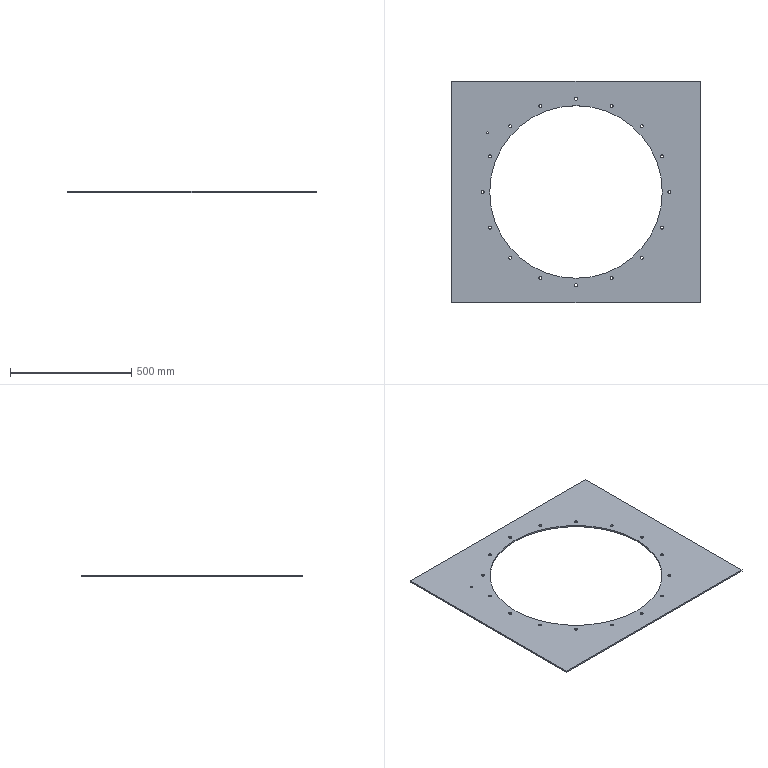Part | STEP file | 750078200 | 1 solid | 42 faces | box 1025 x 915 x 6 mm | volume 3220443 mm3 | cylinder 36 | plane 6 | commonest cylinder face diameters 12 x32 8.2 x2 713 x2
STEP:
#1=CARTESIAN_POINT('',(-356.5,0.,0.));
#2=VERTEX_POINT('',#1);
#3=CARTESIAN_POINT('',(356.5,0.,0.));
#4=VERTEX_POINT('',#3);
#5=CARTESIAN_POINT('',(0.,0.,0.));
#6=DIRECTION('',(0.,0.,1.));
#7=DIRECTION('',(1.,0.,0.));
#8=AXIS2_PLACEMENT_3D('',#5,#6,#7);
#9=CIRCLE('',#8,356.5);
#10=EDGE_CURVE('',#2,#4,#9,.T.);
#11=ORIENTED_EDGE('',*,*,#10,.F.);
#12=CARTESIAN_POINT('',(-356.5,0.,6.));
#13=VERTEX_POINT('',#12);
#14=CARTESIAN_POINT('',(-356.5,0.,-1368.004));
#15=DIRECTION('',(0.,0.,1.));
#16=VECTOR('',#15,1000.);
#17=LINE('',#14,#16);
#18=EDGE_CURVE('',#2,#13,#17,.T.);
#19=ORIENTED_EDGE('',*,*,#18,.T.);
#20=CARTESIAN_POINT('',(356.5,0.,6.));
#21=VERTEX_POINT('',#20);
#22=CARTESIAN_POINT('',(0.,0.,6.));
#23=DIRECTION('',(0.,0.,-1.));
#24=DIRECTION('',(1.,0.,0.));
#25=AXIS2_PLACEMENT_3D('',#22,#23,#24);
#26=CIRCLE('',#25,356.5);
#27=EDGE_CURVE('',#21,#13,#26,.T.);
#28=ORIENTED_EDGE('',*,*,#27,.F.);
#29=CARTESIAN_POINT('',(356.5,0.,-1368.004));
#30=DIRECTION('',(0.,0.,1.));
#31=VECTOR('',#30,1000.);
#32=LINE('',#29,#31);
#33=EDGE_CURVE('',#4,#21,#32,.T.);
#34=ORIENTED_EDGE('',*,*,#33,.F.);
#35=EDGE_LOOP('',(#11,#19,#28,#34));
#36=FACE_OUTER_BOUND('',#35,.T.);
#37=CARTESIAN_POINT('',(0.,0.,-1368.004));
#38=DIRECTION('',(0.,0.,1.));
#39=DIRECTION('',(1.,0.,0.));
#40=AXIS2_PLACEMENT_3D('',#37,#38,#39);
#41=CYLINDRICAL_SURFACE('',#40,356.5);
#42=ADVANCED_FACE('',(#36),#41,.F.);
#43=CARTESIAN_POINT('',(379.,0.,0.));
#44=VERTEX_POINT('',#43);
#45=CARTESIAN_POINT('',(391.,0.,0.));
#46=VERTEX_POINT('',#45);
#47=CARTESIAN_POINT('',(385.,0.,0.));
#48=DIRECTION('',(0.,0.,1.));
#49=DIRECTION('',(1.,0.,0.));
#50=AXIS2_PLACEMENT_3D('',#47,#48,#49);
#51=CIRCLE('',#50,6.);
#52=EDGE_CURVE('',#44,#46,#51,.T.);
#53=ORIENTED_EDGE('',*,*,#52,.F.);
#54=CARTESIAN_POINT('',(379.,0.,6.));
#55=VERTEX_POINT('',#54);
#56=CARTESIAN_POINT('',(379.,0.,-1368.004));
#57=DIRECTION('',(0.,0.,1.));
#58=VECTOR('',#57,1000.);
#59=LINE('',#56,#58);
#60=EDGE_CURVE('',#44,#55,#59,.T.);
#61=ORIENTED_EDGE('',*,*,#60,.T.);
#62=CARTESIAN_POINT('',(391.,0.,6.));
#63=VERTEX_POINT('',#62);
#64=CARTESIAN_POINT('',(385.,0.,6.));
#65=DIRECTION('',(0.,0.,-1.));
#66=DIRECTION('',(1.,0.,0.));
#67=AXIS2_PLACEMENT_3D('',#64,#65,#66);
#68=CIRCLE('',#67,6.);
#69=EDGE_CURVE('',#63,#55,#68,.T.);
#70=ORIENTED_EDGE('',*,*,#69,.F.);
#71=CARTESIAN_POINT('',(391.,0.,-1368.004));
#72=DIRECTION('',(0.,0.,1.));
#73=VECTOR('',#72,1000.);
#74=LINE('',#71,#73);
#75=EDGE_CURVE('',#46,#63,#74,.T.);
#76=ORIENTED_EDGE('',*,*,#75,.F.);
#77=EDGE_LOOP('',(#53,#61,#70,#76));
#78=FACE_OUTER_BOUND('',#77,.T.);
#79=CARTESIAN_POINT('',(385.,0.,-1368.004));
#80=DIRECTION('',(0.,0.,1.));
#81=DIRECTION('',(1.,0.,0.));
#82=AXIS2_PLACEMENT_3D('',#79,#80,#81);
#83=CYLINDRICAL_SURFACE('',#82,6.);
#84=ADVANCED_FACE('',(#78),#83,.F.);
#85=CARTESIAN_POINT('',(349.694,-147.333,0.));
#86=VERTEX_POINT('',#85);
#87=CARTESIAN_POINT('',(361.694,-147.333,0.));
#88=VERTEX_POINT('',#87);
#89=CARTESIAN_POINT('',(355.694,-147.333,0.));
#90=DIRECTION('',(0.,0.,1.));
#91=DIRECTION('',(1.,0.,0.));
#92=AXIS2_PLACEMENT_3D('',#89,#90,#91);
#93=CIRCLE('',#92,6.);
#94=EDGE_CURVE('',#86,#88,#93,.T.);
#95=ORIENTED_EDGE('',*,*,#94,.F.);
#96=CARTESIAN_POINT('',(349.694,-147.333,6.));
#97=VERTEX_POINT('',#96);
#98=CARTESIAN_POINT('',(349.694,-147.333,-1368.004));
#99=DIRECTION('',(0.,0.,1.));
#100=VECTOR('',#99,1000.);
#101=LINE('',#98,#100);
#102=EDGE_CURVE('',#86,#97,#101,.T.);
#103=ORIENTED_EDGE('',*,*,#102,.T.);
#104=CARTESIAN_POINT('',(361.694,-147.333,6.));
#105=VERTEX_POINT('',#104);
#106=CARTESIAN_POINT('',(355.694,-147.333,6.));
#107=DIRECTION('',(0.,0.,-1.));
#108=DIRECTION('',(1.,0.,0.));
#109=AXIS2_PLACEMENT_3D('',#106,#107,#108);
#110=CIRCLE('',#109,6.);
#111=EDGE_CURVE('',#105,#97,#110,.T.);
#112=ORIENTED_EDGE('',*,*,#111,.F.);
#113=CARTESIAN_POINT('',(361.694,-147.333,-1368.004));
#114=DIRECTION('',(0.,0.,1.));
#115=VECTOR('',#114,1000.);
#116=LINE('',#113,#115);
#117=EDGE_CURVE('',#88,#105,#116,.T.);
#118=ORIENTED_EDGE('',*,*,#117,.F.);
#119=EDGE_LOOP('',(#95,#103,#112,#118));
#120=FACE_OUTER_BOUND('',#119,.T.);
#121=CARTESIAN_POINT('',(355.694,-147.333,-1368.004));
#122=DIRECTION('',(0.,0.,1.));
#123=DIRECTION('',(1.,0.,0.));
#124=AXIS2_PLACEMENT_3D('',#121,#122,#123);
#125=CYLINDRICAL_SURFACE('',#124,6.);
#126=ADVANCED_FACE('',(#120),#125,.F.);
#127=CARTESIAN_POINT('',(349.694,147.333,0.));
#128=VERTEX_POINT('',#127);
#129=CARTESIAN_POINT('',(361.694,147.333,0.));
#130=VERTEX_POINT('',#129);
#131=CARTESIAN_POINT('',(355.694,147.333,0.));
#132=DIRECTION('',(0.,0.,1.));
#133=DIRECTION('',(1.,0.,0.));
#134=AXIS2_PLACEMENT_3D('',#131,#132,#133);
#135=CIRCLE('',#134,6.);
#136=EDGE_CURVE('',#128,#130,#135,.T.);
#137=ORIENTED_EDGE('',*,*,#136,.F.);
#138=CARTESIAN_POINT('',(349.694,147.333,6.));
#139=VERTEX_POINT('',#138);
#140=CARTESIAN_POINT('',(349.694,147.333,-1368.004));
#141=DIRECTION('',(0.,0.,1.));
#142=VECTOR('',#141,1000.);
#143=LINE('',#140,#142);
#144=EDGE_CURVE('',#128,#139,#143,.T.);
#145=ORIENTED_EDGE('',*,*,#144,.T.);
#146=CARTESIAN_POINT('',(361.694,147.333,6.));
#147=VERTEX_POINT('',#146);
#148=CARTESIAN_POINT('',(355.694,147.333,6.));
#149=DIRECTION('',(0.,0.,-1.));
#150=DIRECTION('',(1.,0.,0.));
#151=AXIS2_PLACEMENT_3D('',#148,#149,#150);
#152=CIRCLE('',#151,6.);
#153=EDGE_CURVE('',#147,#139,#152,.T.);
#154=ORIENTED_EDGE('',*,*,#153,.F.);
#155=CARTESIAN_POINT('',(361.694,147.333,-1368.004));
#156=DIRECTION('',(0.,0.,1.));
#157=VECTOR('',#156,1000.);
#158=LINE('',#155,#157);
#159=EDGE_CURVE('',#130,#147,#158,.T.);
#160=ORIENTED_EDGE('',*,*,#159,.F.);
#161=EDGE_LOOP('',(#137,#145,#154,#160));
#162=FACE_OUTER_BOUND('',#161,.T.);
#163=CARTESIAN_POINT('',(355.694,147.333,-1368.004));
#164=DIRECTION('',(0.,0.,1.));
#165=DIRECTION('',(1.,0.,0.));
#166=AXIS2_PLACEMENT_3D('',#163,#164,#165);
#167=CYLINDRICAL_SURFACE('',#166,6.);
#168=ADVANCED_FACE('',(#162),#167,.F.);
#169=CARTESIAN_POINT('',(266.236,272.236,0.));
#170=VERTEX_POINT('',#169);
#171=CARTESIAN_POINT('',(278.236,272.236,0.));
#172=VERTEX_POINT('',#171);
#173=CARTESIAN_POINT('',(272.236,272.236,0.));
#174=DIRECTION('',(0.,0.,1.));
#175=DIRECTION('',(1.,0.,0.));
#176=AXIS2_PLACEMENT_3D('',#173,#174,#175);
#177=CIRCLE('',#176,6.);
#178=EDGE_CURVE('',#170,#172,#177,.T.);
#179=ORIENTED_EDGE('',*,*,#178,.F.);
#180=CARTESIAN_POINT('',(266.236,272.236,6.));
#181=VERTEX_POINT('',#180);
#182=CARTESIAN_POINT('',(266.236,272.236,-1368.004));
#183=DIRECTION('',(0.,0.,1.));
#184=VECTOR('',#183,1000.);
#185=LINE('',#182,#184);
#186=EDGE_CURVE('',#170,#181,#185,.T.);
#187=ORIENTED_EDGE('',*,*,#186,.T.);
#188=CARTESIAN_POINT('',(278.236,272.236,6.));
#189=VERTEX_POINT('',#188);
#190=CARTESIAN_POINT('',(272.236,272.236,6.));
#191=DIRECTION('',(0.,0.,-1.));
#192=DIRECTION('',(1.,0.,0.));
#193=AXIS2_PLACEMENT_3D('',#190,#191,#192);
#194=CIRCLE('',#193,6.);
#195=EDGE_CURVE('',#189,#181,#194,.T.);
#196=ORIENTED_EDGE('',*,*,#195,.F.);
#197=CARTESIAN_POINT('',(278.236,272.236,-1368.004));
#198=DIRECTION('',(0.,0.,1.));
#199=VECTOR('',#198,1000.);
#200=LINE('',#197,#199);
#201=EDGE_CURVE('',#172,#189,#200,.T.);
#202=ORIENTED_EDGE('',*,*,#201,.F.);
#203=EDGE_LOOP('',(#179,#187,#196,#202));
#204=FACE_OUTER_BOUND('',#203,.T.);
#205=CARTESIAN_POINT('',(272.236,272.236,-1368.004));
#206=DIRECTION('',(0.,0.,1.));
#207=DIRECTION('',(1.,0.,0.));
#208=AXIS2_PLACEMENT_3D('',#205,#206,#207);
#209=CYLINDRICAL_SURFACE('',#208,6.);
#210=ADVANCED_FACE('',(#204),#209,.F.);
#211=CARTESIAN_POINT('',(266.236,-272.236,0.));
#212=VERTEX_POINT('',#211);
#213=CARTESIAN_POINT('',(278.236,-272.236,0.));
#214=VERTEX_POINT('',#213);
#215=CARTESIAN_POINT('',(272.236,-272.236,0.));
#216=DIRECTION('',(0.,0.,1.));
#217=DIRECTION('',(1.,0.,0.));
#218=AXIS2_PLACEMENT_3D('',#215,#216,#217);
#219=CIRCLE('',#218,6.);
#220=EDGE_CURVE('',#212,#214,#219,.T.);
#221=ORIENTED_EDGE('',*,*,#220,.F.);
#222=CARTESIAN_POINT('',(266.236,-272.236,6.));
#223=VERTEX_POINT('',#222);
#224=CARTESIAN_POINT('',(266.236,-272.236,-1368.004));
#225=DIRECTION('',(0.,0.,1.));
#226=VECTOR('',#225,1000.);
#227=LINE('',#224,#226);
#228=EDGE_CURVE('',#212,#223,#227,.T.);
#229=ORIENTED_EDGE('',*,*,#228,.T.);
#230=CARTESIAN_POINT('',(278.236,-272.236,6.));
#231=VERTEX_POINT('',#230);
#232=CARTESIAN_POINT('',(272.236,-272.236,6.));
#233=DIRECTION('',(0.,0.,-1.));
#234=DIRECTION('',(1.,0.,0.));
#235=AXIS2_PLACEMENT_3D('',#232,#233,#234);
#236=CIRCLE('',#235,6.);
#237=EDGE_CURVE('',#231,#223,#236,.T.);
#238=ORIENTED_EDGE('',*,*,#237,.F.);
#239=CARTESIAN_POINT('',(278.236,-272.236,-1368.004));
#240=DIRECTION('',(0.,0.,1.));
#241=VECTOR('',#240,1000.);
#242=LINE('',#239,#241);
#243=EDGE_CURVE('',#214,#231,#242,.T.);
#244=ORIENTED_EDGE('',*,*,#243,.F.);
#245=EDGE_LOOP('',(#221,#229,#238,#244));
#246=FACE_OUTER_BOUND('',#245,.T.);
#247=CARTESIAN_POINT('',(272.236,-272.236,-1368.004));
#248=DIRECTION('',(0.,0.,1.));
#249=DIRECTION('',(1.,0.,0.));
#250=AXIS2_PLACEMENT_3D('',#247,#248,#249);
#251=CYLINDRICAL_SURFACE('',#250,6.);
#252=ADVANCED_FACE('',(#246),#251,.F.);
#253=CARTESIAN_POINT('',(141.333,355.694,0.));
#254=VERTEX_POINT('',#253);
#255=CARTESIAN_POINT('',(153.333,355.694,0.));
#256=VERTEX_POINT('',#255);
#257=CARTESIAN_POINT('',(147.333,355.694,0.));
#258=DIRECTION('',(0.,0.,1.));
#259=DIRECTION('',(1.,0.,0.));
#260=AXIS2_PLACEMENT_3D('',#257,#258,#259);
#261=CIRCLE('',#260,6.);
#262=EDGE_CURVE('',#254,#256,#261,.T.);
#263=ORIENTED_EDGE('',*,*,#262,.F.);
#264=CARTESIAN_POINT('',(141.333,355.694,6.));
#265=VERTEX_POINT('',#264);
#266=CARTESIAN_POINT('',(141.333,355.694,-1368.004));
#267=DIRECTION('',(0.,0.,1.));
#268=VECTOR('',#267,1000.);
#269=LINE('',#266,#268);
#270=EDGE_CURVE('',#254,#265,#269,.T.);
#271=ORIENTED_EDGE('',*,*,#270,.T.);
#272=CARTESIAN_POINT('',(153.333,355.694,6.));
#273=VERTEX_POINT('',#272);
#274=CARTESIAN_POINT('',(147.333,355.694,6.));
#275=DIRECTION('',(0.,0.,-1.));
#276=DIRECTION('',(1.,0.,0.));
#277=AXIS2_PLACEMENT_3D('',#274,#275,#276);
#278=CIRCLE('',#277,6.);
#279=EDGE_CURVE('',#273,#265,#278,.T.);
#280=ORIENTED_EDGE('',*,*,#279,.F.);
#281=CARTESIAN_POINT('',(153.333,355.694,-1368.004));
#282=DIRECTION('',(0.,0.,1.));
#283=VECTOR('',#282,1000.);
#284=LINE('',#281,#283);
#285=EDGE_CURVE('',#256,#273,#284,.T.);
#286=ORIENTED_EDGE('',*,*,#285,.F.);
#287=EDGE_LOOP('',(#263,#271,#280,#286));
#288=FACE_OUTER_BOUND('',#287,.T.);
#289=CARTESIAN_POINT('',(147.333,355.694,-1368.004));
#290=DIRECTION('',(0.,0.,1.));
#291=DIRECTION('',(1.,0.,0.));
#292=AXIS2_PLACEMENT_3D('',#289,#290,#291);
#293=CYLINDRICAL_SURFACE('',#292,6.);
#294=ADVANCED_FACE('',(#288),#293,.F.);
#295=CARTESIAN_POINT('',(141.333,-355.694,0.));
#296=VERTEX_POINT('',#295);
#297=CARTESIAN_POINT('',(153.333,-355.694,0.));
#298=VERTEX_POINT('',#297);
#299=CARTESIAN_POINT('',(147.333,-355.694,0.));
#300=DIRECTION('',(0.,0.,1.));
#301=DIRECTION('',(1.,0.,0.));
#302=AXIS2_PLACEMENT_3D('',#299,#300,#301);
#303=CIRCLE('',#302,6.);
#304=EDGE_CURVE('',#296,#298,#303,.T.);
#305=ORIENTED_EDGE('',*,*,#304,.F.);
#306=CARTESIAN_POINT('',(141.333,-355.694,6.));
#307=VERTEX_POINT('',#306);
#308=CARTESIAN_POINT('',(141.333,-355.694,-1368.004));
#309=DIRECTION('',(0.,0.,1.));
#310=VECTOR('',#309,1000.);
#311=LINE('',#308,#310);
#312=EDGE_CURVE('',#296,#307,#311,.T.);
#313=ORIENTED_EDGE('',*,*,#312,.T.);
#314=CARTESIAN_POINT('',(153.333,-355.694,6.));
#315=VERTEX_POINT('',#314);
#316=CARTESIAN_POINT('',(147.333,-355.694,6.));
#317=DIRECTION('',(0.,0.,-1.));
#318=DIRECTION('',(1.,0.,0.));
#319=AXIS2_PLACEMENT_3D('',#316,#317,#318);
#320=CIRCLE('',#319,6.);
#321=EDGE_CURVE('',#315,#307,#320,.T.);
#322=ORIENTED_EDGE('',*,*,#321,.F.);
#323=CARTESIAN_POINT('',(153.333,-355.694,-1368.004));
#324=DIRECTION('',(0.,0.,1.));
#325=VECTOR('',#324,1000.);
#326=LINE('',#323,#325);
#327=EDGE_CURVE('',#298,#315,#326,.T.);
#328=ORIENTED_EDGE('',*,*,#327,.F.);
#329=EDGE_LOOP('',(#305,#313,#322,#328));
#330=FACE_OUTER_BOUND('',#329,.T.);
#331=CARTESIAN_POINT('',(147.333,-355.694,-1368.004));
#332=DIRECTION('',(0.,0.,1.));
#333=DIRECTION('',(1.,0.,0.));
#334=AXIS2_PLACEMENT_3D('',#331,#332,#333);
#335=CYLINDRICAL_SURFACE('',#334,6.);
#336=ADVANCED_FACE('',(#330),#335,.F.);
#337=CARTESIAN_POINT('',(-6.,-385.,0.));
#338=VERTEX_POINT('',#337);
#339=CARTESIAN_POINT('',(6.,-385.,0.));
#340=VERTEX_POINT('',#339);
#341=CARTESIAN_POINT('',(0.,-385.,0.));
#342=DIRECTION('',(0.,0.,1.));
#343=DIRECTION('',(1.,0.,0.));
#344=AXIS2_PLACEMENT_3D('',#341,#342,#343);
#345=CIRCLE('',#344,6.);
#346=EDGE_CURVE('',#338,#340,#345,.T.);
#347=ORIENTED_EDGE('',*,*,#346,.F.);
#348=CARTESIAN_POINT('',(-6.,-385.,6.));
#349=VERTEX_POINT('',#348);
#350=CARTESIAN_POINT('',(-6.,-385.,-1368.004));
#351=DIRECTION('',(0.,0.,1.));
#352=VECTOR('',#351,1000.);
#353=LINE('',#350,#352);
#354=EDGE_CURVE('',#338,#349,#353,.T.);
#355=ORIENTED_EDGE('',*,*,#354,.T.);
#356=CARTESIAN_POINT('',(6.,-385.,6.));
#357=VERTEX_POINT('',#356);
#358=CARTESIAN_POINT('',(0.,-385.,6.));
#359=DIRECTION('',(0.,0.,-1.));
#360=DIRECTION('',(1.,0.,0.));
#361=AXIS2_PLACEMENT_3D('',#358,#359,#360);
#362=CIRCLE('',#361,6.);
#363=EDGE_CURVE('',#357,#349,#362,.T.);
#364=ORIENTED_EDGE('',*,*,#363,.F.);
#365=CARTESIAN_POINT('',(6.,-385.,-1368.004));
#366=DIRECTION('',(0.,0.,1.));
#367=VECTOR('',#366,1000.);
#368=LINE('',#365,#367);
#369=EDGE_CURVE('',#340,#357,#368,.T.);
#370=ORIENTED_EDGE('',*,*,#369,.F.);
#371=EDGE_LOOP('',(#347,#355,#364,#370));
#372=FACE_OUTER_BOUND('',#371,.T.);
#373=CARTESIAN_POINT('',(0.,-385.,-1368.004));
#374=DIRECTION('',(0.,0.,1.));
#375=DIRECTION('',(1.,0.,0.));
#376=AXIS2_PLACEMENT_3D('',#373,#374,#375);
#377=CYLINDRICAL_SURFACE('',#376,6.);
#378=ADVANCED_FACE('',(#372),#377,.F.);
#379=CARTESIAN_POINT('',(-6.,385.,0.));
#380=VERTEX_POINT('',#379);
#381=CARTESIAN_POINT('',(6.,385.,0.));
#382=VERTEX_POINT('',#381);
#383=CARTESIAN_POINT('',(0.,385.,0.));
#384=DIRECTION('',(0.,0.,1.));
#385=DIRECTION('',(1.,0.,0.));
#386=AXIS2_PLACEMENT_3D('',#383,#384,#385);
#387=CIRCLE('',#386,6.);
#388=EDGE_CURVE('',#380,#382,#387,.T.);
#389=ORIENTED_EDGE('',*,*,#388,.F.);
#390=CARTESIAN_POINT('',(-6.,385.,6.));
#391=VERTEX_POINT('',#390);
#392=CARTESIAN_POINT('',(-6.,385.,-1368.004));
#393=DIRECTION('',(0.,0.,1.));
#394=VECTOR('',#393,1000.);
#395=LINE('',#392,#394);
#396=EDGE_CURVE('',#380,#391,#395,.T.);
#397=ORIENTED_EDGE('',*,*,#396,.T.);
#398=CARTESIAN_POINT('',(6.,385.,6.));
#399=VERTEX_POINT('',#398);
#400=CARTESIAN_POINT('',(0.,385.,6.));
#401=DIRECTION('',(0.,0.,-1.));
#402=DIRECTION('',(1.,0.,0.));
#403=AXIS2_PLACEMENT_3D('',#400,#401,#402);
#404=CIRCLE('',#403,6.);
#405=EDGE_CURVE('',#399,#391,#404,.T.);
#406=ORIENTED_EDGE('',*,*,#405,.F.);
#407=CARTESIAN_POINT('',(6.,385.,-1368.004));
#408=DIRECTION('',(0.,0.,1.));
#409=VECTOR('',#408,1000.);
#410=LINE('',#407,#409);
#411=EDGE_CURVE('',#382,#399,#410,.T.);
#412=ORIENTED_EDGE('',*,*,#411,.F.);
#413=EDGE_LOOP('',(#389,#397,#406,#412));
#414=FACE_OUTER_BOUND('',#413,.T.);
#415=CARTESIAN_POINT('',(0.,385.,-1368.004));
#416=DIRECTION('',(0.,0.,1.));
#417=DIRECTION('',(1.,0.,0.));
#418=AXIS2_PLACEMENT_3D('',#415,#416,#417);
#419=CYLINDRICAL_SURFACE('',#418,6.);
#420=ADVANCED_FACE('',(#414),#419,.F.);
#421=CARTESIAN_POINT('',(-153.333,355.694,0.));
#422=VERTEX_POINT('',#421);
#423=CARTESIAN_POINT('',(-141.333,355.694,0.));
#424=VERTEX_POINT('',#423);
#425=CARTESIAN_POINT('',(-147.333,355.694,0.));
#426=DIRECTION('',(0.,0.,1.));
#427=DIRECTION('',(1.,0.,0.));
#428=AXIS2_PLACEMENT_3D('',#425,#426,#427);
#429=CIRCLE('',#428,6.);
#430=EDGE_CURVE('',#422,#424,#429,.T.);
#431=ORIENTED_EDGE('',*,*,#430,.F.);
#432=CARTESIAN_POINT('',(-153.333,355.694,6.));
#433=VERTEX_POINT('',#432);
#434=CARTESIAN_POINT('',(-153.333,355.694,-1368.004));
#435=DIRECTION('',(0.,0.,1.));
#436=VECTOR('',#435,1000.);
#437=LINE('',#434,#436);
#438=EDGE_CURVE('',#422,#433,#437,.T.);
#439=ORIENTED_EDGE('',*,*,#438,.T.);
#440=CARTESIAN_POINT('',(-141.333,355.694,6.));
#441=VERTEX_POINT('',#440);
#442=CARTESIAN_POINT('',(-147.333,355.694,6.));
#443=DIRECTION('',(0.,0.,-1.));
#444=DIRECTION('',(1.,0.,0.));
#445=AXIS2_PLACEMENT_3D('',#442,#443,#444);
#446=CIRCLE('',#445,6.);
#447=EDGE_CURVE('',#441,#433,#446,.T.);
#448=ORIENTED_EDGE('',*,*,#447,.F.);
#449=CARTESIAN_POINT('',(-141.333,355.694,-1368.004));
#450=DIRECTION('',(0.,0.,1.));
#451=VECTOR('',#450,1000.);
#452=LINE('',#449,#451);
#453=EDGE_CURVE('',#424,#441,#452,.T.);
#454=ORIENTED_EDGE('',*,*,#453,.F.);
#455=EDGE_LOOP('',(#431,#439,#448,#454));
#456=FACE_OUTER_BOUND('',#455,.T.);
#457=CARTESIAN_POINT('',(-147.333,355.694,-1368.004));
#458=DIRECTION('',(0.,0.,1.));
#459=DIRECTION('',(1.,0.,0.));
#460=AXIS2_PLACEMENT_3D('',#457,#458,#459);
#461=CYLINDRICAL_SURFACE('',#460,6.);
#462=ADVANCED_FACE('',(#456),#461,.F.);
#463=CARTESIAN_POINT('',(-153.333,-355.694,0.));
#464=VERTEX_POINT('',#463);
#465=CARTESIAN_POINT('',(-141.333,-355.694,0.));
#466=VERTEX_POINT('',#465);
#467=CARTESIAN_POINT('',(-147.333,-355.694,0.));
#468=DIRECTION('',(0.,0.,1.));
#469=DIRECTION('',(1.,0.,0.));
#470=AXIS2_PLACEMENT_3D('',#467,#468,#469);
#471=CIRCLE('',#470,6.);
#472=EDGE_CURVE('',#464,#466,#471,.T.);
#473=ORIENTED_EDGE('',*,*,#472,.F.);
#474=CARTESIAN_POINT('',(-153.333,-355.694,6.));
#475=VERTEX_POINT('',#474);
#476=CARTESIAN_POINT('',(-153.333,-355.694,-1368.004));
#477=DIRECTION('',(0.,0.,1.));
#478=VECTOR('',#477,1000.);
#479=LINE('',#476,#478);
#480=EDGE_CURVE('',#464,#475,#479,.T.);
#481=ORIENTED_EDGE('',*,*,#480,.T.);
#482=CARTESIAN_POINT('',(-141.333,-355.694,6.));
#483=VERTEX_POINT('',#482);
#484=CARTESIAN_POINT('',(-147.333,-355.694,6.));
#485=DIRECTION('',(0.,0.,-1.));
#486=DIRECTION('',(1.,0.,0.));
#487=AXIS2_PLACEMENT_3D('',#484,#485,#486);
#488=CIRCLE('',#487,6.);
#489=EDGE_CURVE('',#483,#475,#488,.T.);
#490=ORIENTED_EDGE('',*,*,#489,.F.);
#491=CARTESIAN_POINT('',(-141.333,-355.694,-1368.004));
#492=DIRECTION('',(0.,0.,1.));
#493=VECTOR('',#492,1000.);
#494=LINE('',#491,#493);
#495=EDGE_CURVE('',#466,#483,#494,.T.);
#496=ORIENTED_EDGE('',*,*,#495,.F.);
#497=EDGE_LOOP('',(#473,#481,#490,#496));
#498=FACE_OUTER_BOUND('',#497,.T.);
#499=CARTESIAN_POINT('',(-147.333,-355.694,-1368.004));
#500=DIRECTION('',(0.,0.,1.));
#501=DIRECTION('',(1.,0.,0.));
#502=AXIS2_PLACEMENT_3D('',#499,#500,#501);
#503=CYLINDRICAL_SURFACE('',#502,6.);
#504=ADVANCED_FACE('',(#498),#503,.F.);
#505=CARTESIAN_POINT('',(-278.236,272.236,0.));
#506=VERTEX_POINT('',#505);
#507=CARTESIAN_POINT('',(-266.236,272.236,0.));
#508=VERTEX_POINT('',#507);
#509=CARTESIAN_POINT('',(-272.236,272.236,0.));
#510=DIRECTION('',(0.,0.,1.));
#511=DIRECTION('',(1.,0.,0.));
#512=AXIS2_PLACEMENT_3D('',#509,#510,#511);
#513=CIRCLE('',#512,6.);
#514=EDGE_CURVE('',#506,#508,#513,.T.);
#515=ORIENTED_EDGE('',*,*,#514,.F.);
#516=CARTESIAN_POINT('',(-278.236,272.236,6.));
#517=VERTEX_POINT('',#516);
#518=CARTESIAN_POINT('',(-278.236,272.236,-1368.004));
#519=DIRECTION('',(0.,0.,1.));
#520=VECTOR('',#519,1000.);
#521=LINE('',#518,#520);
#522=EDGE_CURVE('',#506,#517,#521,.T.);
#523=ORIENTED_EDGE('',*,*,#522,.T.);
#524=CARTESIAN_POINT('',(-266.236,272.236,6.));
#525=VERTEX_POINT('',#524);
#526=CARTESIAN_POINT('',(-272.236,272.236,6.));
#527=DIRECTION('',(0.,0.,-1.));
#528=DIRECTION('',(1.,0.,0.));
#529=AXIS2_PLACEMENT_3D('',#526,#527,#528);
#530=CIRCLE('',#529,6.);
#531=EDGE_CURVE('',#525,#517,#530,.T.);
#532=ORIENTED_EDGE('',*,*,#531,.F.);
#533=CARTESIAN_POINT('',(-266.236,272.236,-1368.004));
#534=DIRECTION('',(0.,0.,1.));
#535=VECTOR('',#534,1000.);
#536=LINE('',#533,#535);
#537=EDGE_CURVE('',#508,#525,#536,.T.);
#538=ORIENTED_EDGE('',*,*,#537,.F.);
#539=EDGE_LOOP('',(#515,#523,#532,#538));
#540=FACE_OUTER_BOUND('',#539,.T.);
#541=CARTESIAN_POINT('',(-272.236,272.236,-1368.004));
#542=DIRECTION('',(0.,0.,1.));
#543=DIRECTION('',(1.,0.,0.));
#544=AXIS2_PLACEMENT_3D('',#541,#542,#543);
#545=CYLINDRICAL_SURFACE('',#544,6.);
#546=ADVANCED_FACE('',(#540),#545,.F.);
#547=CARTESIAN_POINT('',(-278.236,-272.236,0.));
#548=VERTEX_POINT('',#547);
#549=CARTESIAN_POINT('',(-266.236,-272.236,0.));
#550=VERTEX_POINT('',#549);
#551=CARTESIAN_POINT('',(-272.236,-272.236,0.));
#552=DIRECTION('',(0.,0.,1.));
#553=DIRECTION('',(1.,0.,0.));
#554=AXIS2_PLACEMENT_3D('',#551,#552,#553);
#555=CIRCLE('',#554,6.);
#556=EDGE_CURVE('',#548,#550,#555,.T.);
#557=ORIENTED_EDGE('',*,*,#556,.F.);
#558=CARTESIAN_POINT('',(-278.236,-272.236,6.));
#559=VERTEX_POINT('',#558);
#560=CARTESIAN_POINT('',(-278.236,-272.236,-1368.004));
#561=DIRECTION('',(0.,0.,1.));
#562=VECTOR('',#561,1000.);
#563=LINE('',#560,#562);
#564=EDGE_CURVE('',#548,#559,#563,.T.);
#565=ORIENTED_EDGE('',*,*,#564,.T.);
#566=CARTESIAN_POINT('',(-266.236,-272.236,6.));
#567=VERTEX_POINT('',#566);
#568=CARTESIAN_POINT('',(-272.236,-272.236,6.));
#569=DIRECTION('',(0.,0.,-1.));
#570=DIRECTION('',(1.,0.,0.));
#571=AXIS2_PLACEMENT_3D('',#568,#569,#570);
#572=CIRCLE('',#571,6.);
#573=EDGE_CURVE('',#567,#559,#572,.T.);
#574=ORIENTED_EDGE('',*,*,#573,.F.);
#575=CARTESIAN_POINT('',(-266.236,-272.236,-1368.004));
#576=DIRECTION('',(0.,0.,1.));
#577=VECTOR('',#576,1000.);
#578=LINE('',#575,#577);
#579=EDGE_CURVE('',#550,#567,#578,.T.);
#580=ORIENTED_EDGE('',*,*,#579,.F.);
#581=EDGE_LOOP('',(#557,#565,#574,#580));
#582=FACE_OUTER_BOUND('',#581,.T.);
#583=CARTESIAN_POINT('',(-272.236,-272.236,-1368.004));
#584=DIRECTION('',(0.,0.,1.));
#585=DIRECTION('',(1.,0.,0.));
#586=AXIS2_PLACEMENT_3D('',#583,#584,#585);
#587=CYLINDRICAL_SURFACE('',#586,6.);
#588=ADVANCED_FACE('',(#582),#587,.F.);
#589=CARTESIAN_POINT('',(-361.694,-147.333,0.));
#590=VERTEX_POINT('',#589);
#591=CARTESIAN_POINT('',(-349.694,-147.333,0.));
#592=VERTEX_POINT('',#591);
#593=CARTESIAN_POINT('',(-355.694,-147.333,0.));
#594=DIRECTION('',(0.,0.,1.));
#595=DIRECTION('',(1.,0.,0.));
#596=AXIS2_PLACEMENT_3D('',#593,#594,#595);
#597=CIRCLE('',#596,6.);
#598=EDGE_CURVE('',#590,#592,#597,.T.);
#599=ORIENTED_EDGE('',*,*,#598,.F.);
#600=CARTESIAN_POINT('',(-361.694,-147.333,6.));
#601=VERTEX_POINT('',#600);
#602=CARTESIAN_POINT('',(-361.694,-147.333,-1368.004));
#603=DIRECTION('',(0.,0.,1.));
#604=VECTOR('',#603,1000.);
#605=LINE('',#602,#604);
#606=EDGE_CURVE('',#590,#601,#605,.T.);
#607=ORIENTED_EDGE('',*,*,#606,.T.);
#608=CARTESIAN_POINT('',(-349.694,-147.333,6.));
#609=VERTEX_POINT('',#608);
#610=CARTESIAN_POINT('',(-355.694,-147.333,6.));
#611=DIRECTION('',(0.,0.,-1.));
#612=DIRECTION('',(1.,0.,0.));
#613=AXIS2_PLACEMENT_3D('',#610,#611,#612);
#614=CIRCLE('',#613,6.);
#615=EDGE_CURVE('',#609,#601,#614,.T.);
#616=ORIENTED_EDGE('',*,*,#615,.F.);
#617=CARTESIAN_POINT('',(-349.694,-147.333,-1368.004));
#618=DIRECTION('',(0.,0.,1.));
#619=VECTOR('',#618,1000.);
#620=LINE('',#617,#619);
#621=EDGE_CURVE('',#592,#609,#620,.T.);
#622=ORIENTED_EDGE('',*,*,#621,.F.);
#623=EDGE_LOOP('',(#599,#607,#616,#622));
#624=FACE_OUTER_BOUND('',#623,.T.);
#625=CARTESIAN_POINT('',(-355.694,-147.333,-1368.004));
#626=DIRECTION('',(0.,0.,1.));
#627=DIRECTION('',(1.,0.,0.));
#628=AXIS2_PLACEMENT_3D('',#625,#626,#627);
#629=CYLINDRICAL_SURFACE('',#628,6.);
#630=ADVANCED_FACE('',(#624),#629,.F.);
#631=CARTESIAN_POINT('',(-361.694,147.333,0.));
#632=VERTEX_POINT('',#631);
#633=CARTESIAN_POINT('',(-349.694,147.333,0.));
#634=VERTEX_POINT('',#633);
#635=CARTESIAN_POINT('',(-355.694,147.333,0.));
#636=DIRECTION('',(0.,0.,1.));
#637=DIRECTION('',(1.,0.,0.));
#638=AXIS2_PLACEMENT_3D('',#635,#636,#637);
#639=CIRCLE('',#638,6.);
#640=EDGE_CURVE('',#632,#634,#639,.T.);
#641=ORIENTED_EDGE('',*,*,#640,.F.);
#642=CARTESIAN_POINT('',(-361.694,147.333,6.));
#643=VERTEX_POINT('',#642);
#644=CARTESIAN_POINT('',(-361.694,147.333,-1368.004));
#645=DIRECTION('',(0.,0.,1.));
#646=VECTOR('',#645,1000.);
#647=LINE('',#644,#646);
#648=EDGE_CURVE('',#632,#643,#647,.T.);
#649=ORIENTED_EDGE('',*,*,#648,.T.);
#650=CARTESIAN_POINT('',(-349.694,147.333,6.));
#651=VERTEX_POINT('',#650);
#652=CARTESIAN_POINT('',(-355.694,147.333,6.));
#653=DIRECTION('',(0.,0.,-1.));
#654=DIRECTION('',(1.,0.,0.));
#655=AXIS2_PLACEMENT_3D('',#652,#653,#654);
#656=CIRCLE('',#655,6.);
#657=EDGE_CURVE('',#651,#643,#656,.T.);
#658=ORIENTED_EDGE('',*,*,#657,.F.);
#659=CARTESIAN_POINT('',(-349.694,147.333,-1368.004));
#660=DIRECTION('',(0.,0.,1.));
#661=VECTOR('',#660,1000.);
#662=LINE('',#659,#661);
#663=EDGE_CURVE('',#634,#651,#662,.T.);
#664=ORIENTED_EDGE('',*,*,#663,.F.);
#665=EDGE_LOOP('',(#641,#649,#658,#664));
#666=FACE_OUTER_BOUND('',#665,.T.);
#667=CARTESIAN_POINT('',(-355.694,147.333,-1368.004));
#668=DIRECTION('',(0.,0.,1.));
#669=DIRECTION('',(1.,0.,0.));
#670=AXIS2_PLACEMENT_3D('',#667,#668,#669);
#671=CYLINDRICAL_SURFACE('',#670,6.);
#672=ADVANCED_FACE('',(#666),#671,.F.);
#673=CARTESIAN_POINT('',(-369.947,244.451,0.));
#674=VERTEX_POINT('',#673);
#675=CARTESIAN_POINT('',(-361.747,244.451,0.));
#676=VERTEX_POINT('',#675);
#677=CARTESIAN_POINT('',(-365.847,244.451,0.));
#678=DIRECTION('',(0.,0.,1.));
#679=DIRECTION('',(1.,0.,0.));
#680=AXIS2_PLACEMENT_3D('',#677,#678,#679);
#681=CIRCLE('',#680,4.1);
#682=EDGE_CURVE('',#674,#676,#681,.T.);
#683=ORIENTED_EDGE('',*,*,#682,.F.);
#684=CARTESIAN_POINT('',(-369.947,244.451,6.));
#685=VERTEX_POINT('',#684);
#686=CARTESIAN_POINT('',(-369.947,244.451,-1368.004));
#687=DIRECTION('',(0.,0.,1.));
#688=VECTOR('',#687,1000.);
#689=LINE('',#686,#688);
#690=EDGE_CURVE('',#674,#685,#689,.T.);
#691=ORIENTED_EDGE('',*,*,#690,.T.);
#692=CARTESIAN_POINT('',(-361.747,244.451,6.));
#693=VERTEX_POINT('',#692);
#694=CARTESIAN_POINT('',(-365.847,244.451,6.));
#695=DIRECTION('',(0.,0.,-1.));
#696=DIRECTION('',(1.,0.,0.));
#697=AXIS2_PLACEMENT_3D('',#694,#695,#696);
#698=CIRCLE('',#697,4.1);
#699=EDGE_CURVE('',#693,#685,#698,.T.);
#700=ORIENTED_EDGE('',*,*,#699,.F.);
#701=CARTESIAN_POINT('',(-361.747,244.451,-1368.004));
#702=DIRECTION('',(0.,0.,1.));
#703=VECTOR('',#702,1000.);
#704=LINE('',#701,#703);
#705=EDGE_CURVE('',#676,#693,#704,.T.);
#706=ORIENTED_EDGE('',*,*,#705,.F.);
#707=EDGE_LOOP('',(#683,#691,#700,#706));
#708=FACE_OUTER_BOUND('',#707,.T.);
#709=CARTESIAN_POINT('',(-365.847,244.451,-1368.004));
#710=DIRECTION('',(0.,0.,1.));
#711=DIRECTION('',(1.,0.,0.));
#712=AXIS2_PLACEMENT_3D('',#709,#710,#711);
#713=CYLINDRICAL_SURFACE('',#712,4.1);
#714=ADVANCED_FACE('',(#708),#713,.F.);
#715=CARTESIAN_POINT('',(-391.,0.,0.));
#716=VERTEX_POINT('',#715);
#717=CARTESIAN_POINT('',(-379.,0.,0.));
#718=VERTEX_POINT('',#717);
#719=CARTESIAN_POINT('',(-385.,0.,0.));
#720=DIRECTION('',(0.,0.,1.));
#721=DIRECTION('',(1.,0.,0.));
#722=AXIS2_PLACEMENT_3D('',#719,#720,#721);
#723=CIRCLE('',#722,6.);
#724=EDGE_CURVE('',#716,#718,#723,.T.);
#725=ORIENTED_EDGE('',*,*,#724,.F.);
#726=CARTESIAN_POINT('',(-391.,0.,6.));
#727=VERTEX_POINT('',#726);
#728=CARTESIAN_POINT('',(-391.,0.,-1368.004));
#729=DIRECTION('',(0.,0.,1.));
#730=VECTOR('',#729,1000.);
#731=LINE('',#728,#730);
#732=EDGE_CURVE('',#716,#727,#731,.T.);
#733=ORIENTED_EDGE('',*,*,#732,.T.);
#734=CARTESIAN_POINT('',(-379.,0.,6.));
#735=VERTEX_POINT('',#734);
#736=CARTESIAN_POINT('',(-385.,0.,6.));
#737=DIRECTION('',(0.,0.,-1.));
#738=DIRECTION('',(1.,0.,0.));
#739=AXIS2_PLACEMENT_3D('',#736,#737,#738);
#740=CIRCLE('',#739,6.);
#741=EDGE_CURVE('',#735,#727,#740,.T.);
#742=ORIENTED_EDGE('',*,*,#741,.F.);
#743=CARTESIAN_POINT('',(-379.,0.,-1368.004));
#744=DIRECTION('',(0.,0.,1.));
#745=VECTOR('',#744,1000.);
#746=LINE('',#743,#745);
#747=EDGE_CURVE('',#718,#735,#746,.T.);
#748=ORIENTED_EDGE('',*,*,#747,.F.);
#749=EDGE_LOOP('',(#725,#733,#742,#748));
#750=FACE_OUTER_BOUND('',#749,.T.);
#751=CARTESIAN_POINT('',(-385.,0.,-1368.004));
#752=DIRECTION('',(0.,0.,1.));
#753=DIRECTION('',(1.,0.,0.));
#754=AXIS2_PLACEMENT_3D('',#751,#752,#753);
#755=CYLINDRICAL_SURFACE('',#754,6.);
#756=ADVANCED_FACE('',(#750),#755,.F.);
#757=CARTESIAN_POINT('',(-512.5,-457.5,6.));
#758=VERTEX_POINT('',#757);
#759=CARTESIAN_POINT('',(512.5,-457.5,6.));
#760=VERTEX_POINT('',#759);
#761=CARTESIAN_POINT('',(0.,-457.5,6.));
#762=DIRECTION('',(1.,0.,0.));
#763=VECTOR('',#762,1000.);
#764=LINE('',#761,#763);
#765=EDGE_CURVE('',#758,#760,#764,.T.);
#766=ORIENTED_EDGE('',*,*,#765,.T.);
#767=CARTESIAN_POINT('',(512.5,457.5,6.));
#768=VERTEX_POINT('',#767);
#769=CARTESIAN_POINT('',(512.5,0.,6.));
#770=DIRECTION('',(0.,1.,0.));
#771=VECTOR('',#770,1000.);
#772=LINE('',#769,#771);
#773=EDGE_CURVE('',#760,#768,#772,.T.);
#774=ORIENTED_EDGE('',*,*,#773,.T.);
#775=CARTESIAN_POINT('',(-512.5,457.5,6.));
#776=VERTEX_POINT('',#775);
#777=CARTESIAN_POINT('',(0.,457.5,6.));
#778=DIRECTION('',(-1.,0.,0.));
#779=VECTOR('',#778,1000.);
#780=LINE('',#777,#779);
#781=EDGE_CURVE('',#768,#776,#780,.T.);
#782=ORIENTED_EDGE('',*,*,#781,.T.);
#783=CARTESIAN_POINT('',(-512.5,0.,6.));
#784=DIRECTION('',(0.,-1.,0.));
#785=VECTOR('',#784,1000.);
#786=LINE('',#783,#785);
#787=EDGE_CURVE('',#776,#758,#786,.T.);
#788=ORIENTED_EDGE('',*,*,#787,.T.);
#789=EDGE_LOOP('',(#766,#774,#782,#788));
#790=FACE_OUTER_BOUND('',#789,.T.);
#791=ORIENTED_EDGE('',*,*,#27,.T.);
#792=CARTESIAN_POINT('',(0.,0.,6.));
#793=DIRECTION('',(0.,0.,-1.));
#794=DIRECTION('',(1.,0.,0.));
#795=AXIS2_PLACEMENT_3D('',#792,#793,#794);
#796=CIRCLE('',#795,356.5);
#797=EDGE_CURVE('',#13,#21,#796,.T.);
#798=ORIENTED_EDGE('',*,*,#797,.T.);
#799=EDGE_LOOP('',(#791,#798));
#800=FACE_BOUND('',#799,.T.);
#801=ORIENTED_EDGE('',*,*,#69,.T.);
#802=CARTESIAN_POINT('',(385.,0.,6.));
#803=DIRECTION('',(0.,0.,-1.));
#804=DIRECTION('',(1.,0.,0.));
#805=AXIS2_PLACEMENT_3D('',#802,#803,#804);
#806=CIRCLE('',#805,6.);
#807=EDGE_CURVE('',#55,#63,#806,.T.);
#808=ORIENTED_EDGE('',*,*,#807,.T.);
#809=EDGE_LOOP('',(#801,#808));
#810=FACE_BOUND('',#809,.T.);
#811=ORIENTED_EDGE('',*,*,#111,.T.);
#812=CARTESIAN_POINT('',(355.694,-147.333,6.));
#813=DIRECTION('',(0.,0.,-1.));
#814=DIRECTION('',(1.,0.,0.));
#815=AXIS2_PLACEMENT_3D('',#812,#813,#814);
#816=CIRCLE('',#815,6.);
#817=EDGE_CURVE('',#97,#105,#816,.T.);
#818=ORIENTED_EDGE('',*,*,#817,.T.);
#819=EDGE_LOOP('',(#811,#818));
#820=FACE_BOUND('',#819,.T.);
#821=ORIENTED_EDGE('',*,*,#153,.T.);
#822=CARTESIAN_POINT('',(355.694,147.333,6.));
#823=DIRECTION('',(0.,0.,-1.));
#824=DIRECTION('',(1.,0.,0.));
#825=AXIS2_PLACEMENT_3D('',#822,#823,#824);
#826=CIRCLE('',#825,6.);
#827=EDGE_CURVE('',#139,#147,#826,.T.);
#828=ORIENTED_EDGE('',*,*,#827,.T.);
#829=EDGE_LOOP('',(#821,#828));
#830=FACE_BOUND('',#829,.T.);
#831=ORIENTED_EDGE('',*,*,#195,.T.);
#832=CARTESIAN_POINT('',(272.236,272.236,6.));
#833=DIRECTION('',(0.,0.,-1.));
#834=DIRECTION('',(1.,0.,0.));
#835=AXIS2_PLACEMENT_3D('',#832,#833,#834);
#836=CIRCLE('',#835,6.);
#837=EDGE_CURVE('',#181,#189,#836,.T.);
#838=ORIENTED_EDGE('',*,*,#837,.T.);
#839=EDGE_LOOP('',(#831,#838));
#840=FACE_BOUND('',#839,.T.);
#841=ORIENTED_EDGE('',*,*,#237,.T.);
#842=CARTESIAN_POINT('',(272.236,-272.236,6.));
#843=DIRECTION('',(0.,0.,-1.));
#844=DIRECTION('',(1.,0.,0.));
#845=AXIS2_PLACEMENT_3D('',#842,#843,#844);
#846=CIRCLE('',#845,6.);
#847=EDGE_CURVE('',#223,#231,#846,.T.);
#848=ORIENTED_EDGE('',*,*,#847,.T.);
#849=EDGE_LOOP('',(#841,#848));
#850=FACE_BOUND('',#849,.T.);
#851=ORIENTED_EDGE('',*,*,#279,.T.);
#852=CARTESIAN_POINT('',(147.333,355.694,6.));
#853=DIRECTION('',(0.,0.,-1.));
#854=DIRECTION('',(1.,0.,0.));
#855=AXIS2_PLACEMENT_3D('',#852,#853,#854);
#856=CIRCLE('',#855,6.);
#857=EDGE_CURVE('',#265,#273,#856,.T.);
#858=ORIENTED_EDGE('',*,*,#857,.T.);
#859=EDGE_LOOP('',(#851,#858));
#860=FACE_BOUND('',#859,.T.);
#861=ORIENTED_EDGE('',*,*,#321,.T.);
#862=CARTESIAN_POINT('',(147.333,-355.694,6.));
#863=DIRECTION('',(0.,0.,-1.));
#864=DIRECTION('',(1.,0.,0.));
#865=AXIS2_PLACEMENT_3D('',#862,#863,#864);
#866=CIRCLE('',#865,6.);
#867=EDGE_CURVE('',#307,#315,#866,.T.);
#868=ORIENTED_EDGE('',*,*,#867,.T.);
#869=EDGE_LOOP('',(#861,#868));
#870=FACE_BOUND('',#869,.T.);
#871=ORIENTED_EDGE('',*,*,#363,.T.);
#872=CARTESIAN_POINT('',(0.,-385.,6.));
#873=DIRECTION('',(0.,0.,-1.));
#874=DIRECTION('',(1.,0.,0.));
#875=AXIS2_PLACEMENT_3D('',#872,#873,#874);
#876=CIRCLE('',#875,6.);
#877=EDGE_CURVE('',#349,#357,#876,.T.);
#878=ORIENTED_EDGE('',*,*,#877,.T.);
#879=EDGE_LOOP('',(#871,#878));
#880=FACE_BOUND('',#879,.T.);
#881=ORIENTED_EDGE('',*,*,#405,.T.);
#882=CARTESIAN_POINT('',(0.,385.,6.));
#883=DIRECTION('',(0.,0.,-1.));
#884=DIRECTION('',(1.,0.,0.));
#885=AXIS2_PLACEMENT_3D('',#882,#883,#884);
#886=CIRCLE('',#885,6.);
#887=EDGE_CURVE('',#391,#399,#886,.T.);
#888=ORIENTED_EDGE('',*,*,#887,.T.);
#889=EDGE_LOOP('',(#881,#888));
#890=FACE_BOUND('',#889,.T.);
#891=ORIENTED_EDGE('',*,*,#447,.T.);
#892=CARTESIAN_POINT('',(-147.333,355.694,6.));
#893=DIRECTION('',(0.,0.,-1.));
#894=DIRECTION('',(1.,0.,0.));
#895=AXIS2_PLACEMENT_3D('',#892,#893,#894);
#896=CIRCLE('',#895,6.);
#897=EDGE_CURVE('',#433,#441,#896,.T.);
#898=ORIENTED_EDGE('',*,*,#897,.T.);
#899=EDGE_LOOP('',(#891,#898));
#900=FACE_BOUND('',#899,.T.);
#901=ORIENTED_EDGE('',*,*,#489,.T.);
#902=CARTESIAN_POINT('',(-147.333,-355.694,6.));
#903=DIRECTION('',(0.,0.,-1.));
#904=DIRECTION('',(1.,0.,0.));
#905=AXIS2_PLACEMENT_3D('',#902,#903,#904);
#906=CIRCLE('',#905,6.);
#907=EDGE_CURVE('',#475,#483,#906,.T.);
#908=ORIENTED_EDGE('',*,*,#907,.T.);
#909=EDGE_LOOP('',(#901,#908));
#910=FACE_BOUND('',#909,.T.);
#911=ORIENTED_EDGE('',*,*,#531,.T.);
#912=CARTESIAN_POINT('',(-272.236,272.236,6.));
#913=DIRECTION('',(0.,0.,-1.));
#914=DIRECTION('',(1.,0.,0.));
#915=AXIS2_PLACEMENT_3D('',#912,#913,#914);
#916=CIRCLE('',#915,6.);
#917=EDGE_CURVE('',#517,#525,#916,.T.);
#918=ORIENTED_EDGE('',*,*,#917,.T.);
#919=EDGE_LOOP('',(#911,#918));
#920=FACE_BOUND('',#919,.T.);
#921=ORIENTED_EDGE('',*,*,#573,.T.);
#922=CARTESIAN_POINT('',(-272.236,-272.236,6.));
#923=DIRECTION('',(0.,0.,-1.));
#924=DIRECTION('',(1.,0.,0.));
#925=AXIS2_PLACEMENT_3D('',#922,#923,#924);
#926=CIRCLE('',#925,6.);
#927=EDGE_CURVE('',#559,#567,#926,.T.);
#928=ORIENTED_EDGE('',*,*,#927,.T.);
#929=EDGE_LOOP('',(#921,#928));
#930=FACE_BOUND('',#929,.T.);
#931=ORIENTED_EDGE('',*,*,#615,.T.);
#932=CARTESIAN_POINT('',(-355.694,-147.333,6.));
#933=DIRECTION('',(0.,0.,-1.));
#934=DIRECTION('',(1.,0.,0.));
#935=AXIS2_PLACEMENT_3D('',#932,#933,#934);
#936=CIRCLE('',#935,6.);
#937=EDGE_CURVE('',#601,#609,#936,.T.);
#938=ORIENTED_EDGE('',*,*,#937,.T.);
#939=EDGE_LOOP('',(#931,#938));
#940=FACE_BOUND('',#939,.T.);
#941=ORIENTED_EDGE('',*,*,#657,.T.);
#942=CARTESIAN_POINT('',(-355.694,147.333,6.));
#943=DIRECTION('',(0.,0.,-1.));
#944=DIRECTION('',(1.,0.,0.));
#945=AXIS2_PLACEMENT_3D('',#942,#943,#944);
#946=CIRCLE('',#945,6.);
#947=EDGE_CURVE('',#643,#651,#946,.T.);
#948=ORIENTED_EDGE('',*,*,#947,.T.);
#949=EDGE_LOOP('',(#941,#948));
#950=FACE_BOUND('',#949,.T.);
#951=ORIENTED_EDGE('',*,*,#699,.T.);
#952=CARTESIAN_POINT('',(-365.847,244.451,6.));
#953=DIRECTION('',(0.,0.,-1.));
#954=DIRECTION('',(1.,0.,0.));
#955=AXIS2_PLACEMENT_3D('',#952,#953,#954);
#956=CIRCLE('',#955,4.1);
#957=EDGE_CURVE('',#685,#693,#956,.T.);
#958=ORIENTED_EDGE('',*,*,#957,.T.);
#959=EDGE_LOOP('',(#951,#958));
#960=FACE_BOUND('',#959,.T.);
#961=ORIENTED_EDGE('',*,*,#741,.T.);
#962=CARTESIAN_POINT('',(-385.,0.,6.));
#963=DIRECTION('',(0.,0.,-1.));
#964=DIRECTION('',(1.,0.,0.));
#965=AXIS2_PLACEMENT_3D('',#962,#963,#964);
#966=CIRCLE('',#965,6.);
#967=EDGE_CURVE('',#727,#735,#966,.T.);
#968=ORIENTED_EDGE('',*,*,#967,.T.);
#969=EDGE_LOOP('',(#961,#968));
#970=FACE_BOUND('',#969,.T.);
#971=CARTESIAN_POINT('',(0.,0.,6.));
#972=DIRECTION('',(0.,0.,1.));
#973=DIRECTION('',(1.,0.,0.));
#974=AXIS2_PLACEMENT_3D('',#971,#972,#973);
#975=PLANE('',#974);
#976=ADVANCED_FACE('',(#790,#800,#810,#820,#830,#840,#850,#860,#870,#880,#890,#900,#910,#920,#930,#940,#950,#960,#970),#975,.T.);
#977=CARTESIAN_POINT('',(512.5,457.5,0.));
#978=VERTEX_POINT('',#977);
#979=CARTESIAN_POINT('',(512.5,457.5,6.));
#980=DIRECTION('',(0.,0.,-1.));
#981=VECTOR('',#980,1000.);
#982=LINE('',#979,#981);
#983=EDGE_CURVE('',#768,#978,#982,.T.);
#984=ORIENTED_EDGE('',*,*,#983,.F.);
#985=ORIENTED_EDGE('',*,*,#773,.F.);
#986=CARTESIAN_POINT('',(512.5,-457.5,0.));
#987=VERTEX_POINT('',#986);
#988=CARTESIAN_POINT('',(512.5,-457.5,6.));
#989=DIRECTION('',(0.,0.,1.));
#990=VECTOR('',#989,1000.);
#991=LINE('',#988,#990);
#992=EDGE_CURVE('',#987,#760,#991,.T.);
#993=ORIENTED_EDGE('',*,*,#992,.F.);
#994=CARTESIAN_POINT('',(512.5,-457.5,0.));
#995=DIRECTION('',(0.,-1.,0.));
#996=VECTOR('',#995,1000.);
#997=LINE('',#994,#996);
#998=EDGE_CURVE('',#978,#987,#997,.T.);
#999=ORIENTED_EDGE('',*,*,#998,.F.);
#1000=EDGE_LOOP('',(#984,#985,#993,#999));
#1001=FACE_OUTER_BOUND('',#1000,.T.);
#1002=CARTESIAN_POINT('',(512.5,-457.5,6.));
#1003=DIRECTION('',(-1.,0.,0.));
#1004=DIRECTION('',(0.,0.,1.));
#1005=AXIS2_PLACEMENT_3D('',#1002,#1003,#1004);
#1006=PLANE('',#1005);
#1007=ADVANCED_FACE('',(#1001),#1006,.F.);
#1008=ORIENTED_EDGE('',*,*,#992,.T.);
#1009=ORIENTED_EDGE('',*,*,#765,.F.);
#1010=CARTESIAN_POINT('',(-512.5,-457.5,0.));
#1011=VERTEX_POINT('',#1010);
#1012=CARTESIAN_POINT('',(-512.5,-457.5,6.));
#1013=DIRECTION('',(0.,0.,1.));
#1014=VECTOR('',#1013,1000.);
#1015=LINE('',#1012,#1014);
#1016=EDGE_CURVE('',#1011,#758,#1015,.T.);
#1017=ORIENTED_EDGE('',*,*,#1016,.F.);
#1018=CARTESIAN_POINT('',(-512.5,-457.5,0.));
#1019=DIRECTION('',(-1.,0.,0.));
#1020=VECTOR('',#1019,1000.);
#1021=LINE('',#1018,#1020);
#1022=EDGE_CURVE('',#987,#1011,#1021,.T.);
#1023=ORIENTED_EDGE('',*,*,#1022,.F.);
#1024=EDGE_LOOP('',(#1008,#1009,#1017,#1023));
#1025=FACE_OUTER_BOUND('',#1024,.T.);
#1026=CARTESIAN_POINT('',(-512.5,-457.5,6.));
#1027=DIRECTION('',(0.,1.,0.));
#1028=DIRECTION('',(0.,0.,1.));
#1029=AXIS2_PLACEMENT_3D('',#1026,#1027,#1028);
#1030=PLANE('',#1029);
#1031=ADVANCED_FACE('',(#1025),#1030,.F.);
#1032=ORIENTED_EDGE('',*,*,#1016,.T.);
#1033=ORIENTED_EDGE('',*,*,#787,.F.);
#1034=CARTESIAN_POINT('',(-512.5,457.5,0.));
#1035=VERTEX_POINT('',#1034);
#1036=CARTESIAN_POINT('',(-512.5,457.5,6.));
#1037=DIRECTION('',(0.,0.,1.));
#1038=VECTOR('',#1037,1000.);
#1039=LINE('',#1036,#1038);
#1040=EDGE_CURVE('',#1035,#776,#1039,.T.);
#1041=ORIENTED_EDGE('',*,*,#1040,.F.);
#1042=CARTESIAN_POINT('',(-512.5,457.5,0.));
#1043=DIRECTION('',(0.,1.,0.));
#1044=VECTOR('',#1043,1000.);
#1045=LINE('',#1042,#1044);
#1046=EDGE_CURVE('',#1011,#1035,#1045,.T.);
#1047=ORIENTED_EDGE('',*,*,#1046,.F.);
#1048=EDGE_LOOP('',(#1032,#1033,#1041,#1047));
#1049=FACE_OUTER_BOUND('',#1048,.T.);
#1050=CARTESIAN_POINT('',(-512.5,457.5,6.));
#1051=DIRECTION('',(1.,0.,0.));
#1052=DIRECTION('',(0.,0.,-1.));
#1053=AXIS2_PLACEMENT_3D('',#1050,#1051,#1052);
#1054=PLANE('',#1053);
#1055=ADVANCED_FACE('',(#1049),#1054,.F.);
#1056=ORIENTED_EDGE('',*,*,#1040,.T.);
#1057=ORIENTED_EDGE('',*,*,#781,.F.);
#1058=ORIENTED_EDGE('',*,*,#983,.T.);
#1059=CARTESIAN_POINT('',(512.5,457.5,0.));
#1060=DIRECTION('',(1.,0.,0.));
#1061=VECTOR('',#1060,1000.);
#1062=LINE('',#1059,#1061);
#1063=EDGE_CURVE('',#1035,#978,#1062,.T.);
#1064=ORIENTED_EDGE('',*,*,#1063,.F.);
#1065=EDGE_LOOP('',(#1056,#1057,#1058,#1064));
#1066=FACE_OUTER_BOUND('',#1065,.T.);
#1067=CARTESIAN_POINT('',(512.5,457.5,6.));
#1068=DIRECTION('',(0.,-1.,0.));
#1069=DIRECTION('',(0.,0.,-1.));
#1070=AXIS2_PLACEMENT_3D('',#1067,#1068,#1069);
#1071=PLANE('',#1070);
#1072=ADVANCED_FACE('',(#1066),#1071,.F.);
#1073=ORIENTED_EDGE('',*,*,#18,.F.);
#1074=CARTESIAN_POINT('',(0.,0.,0.));
#1075=DIRECTION('',(0.,0.,1.));
#1076=DIRECTION('',(1.,0.,0.));
#1077=AXIS2_PLACEMENT_3D('',#1074,#1075,#1076);
#1078=CIRCLE('',#1077,356.5);
#1079=EDGE_CURVE('',#4,#2,#1078,.T.);
#1080=ORIENTED_EDGE('',*,*,#1079,.F.);
#1081=ORIENTED_EDGE('',*,*,#33,.T.);
#1082=ORIENTED_EDGE('',*,*,#797,.F.);
#1083=EDGE_LOOP('',(#1073,#1080,#1081,#1082));
#1084=FACE_OUTER_BOUND('',#1083,.T.);
#1085=CARTESIAN_POINT('',(0.,0.,-1368.004));
#1086=DIRECTION('',(0.,0.,1.));
#1087=DIRECTION('',(1.,0.,0.));
#1088=AXIS2_PLACEMENT_3D('',#1085,#1086,#1087);
#1089=CYLINDRICAL_SURFACE('',#1088,356.5);
#1090=ADVANCED_FACE('',(#1084),#1089,.F.);
#1091=ORIENTED_EDGE('',*,*,#60,.F.);
#1092=CARTESIAN_POINT('',(385.,0.,0.));
#1093=DIRECTION('',(0.,0.,1.));
#1094=DIRECTION('',(1.,0.,0.));
#1095=AXIS2_PLACEMENT_3D('',#1092,#1093,#1094);
#1096=CIRCLE('',#1095,6.);
#1097=EDGE_CURVE('',#46,#44,#1096,.T.);
#1098=ORIENTED_EDGE('',*,*,#1097,.F.);
#1099=ORIENTED_EDGE('',*,*,#75,.T.);
#1100=ORIENTED_EDGE('',*,*,#807,.F.);
#1101=EDGE_LOOP('',(#1091,#1098,#1099,#1100));
#1102=FACE_OUTER_BOUND('',#1101,.T.);
#1103=CARTESIAN_POINT('',(385.,0.,-1368.004));
#1104=DIRECTION('',(0.,0.,1.));
#1105=DIRECTION('',(1.,0.,0.));
#1106=AXIS2_PLACEMENT_3D('',#1103,#1104,#1105);
#1107=CYLINDRICAL_SURFACE('',#1106,6.);
#1108=ADVANCED_FACE('',(#1102),#1107,.F.);
#1109=ORIENTED_EDGE('',*,*,#102,.F.);
#1110=CARTESIAN_POINT('',(355.694,-147.333,0.));
#1111=DIRECTION('',(0.,0.,1.));
#1112=DIRECTION('',(1.,0.,0.));
#1113=AXIS2_PLACEMENT_3D('',#1110,#1111,#1112);
#1114=CIRCLE('',#1113,6.);
#1115=EDGE_CURVE('',#88,#86,#1114,.T.);
#1116=ORIENTED_EDGE('',*,*,#1115,.F.);
#1117=ORIENTED_EDGE('',*,*,#117,.T.);
#1118=ORIENTED_EDGE('',*,*,#817,.F.);
#1119=EDGE_LOOP('',(#1109,#1116,#1117,#1118));
#1120=FACE_OUTER_BOUND('',#1119,.T.);
#1121=CARTESIAN_POINT('',(355.694,-147.333,-1368.004));
#1122=DIRECTION('',(0.,0.,1.));
#1123=DIRECTION('',(1.,0.,0.));
#1124=AXIS2_PLACEMENT_3D('',#1121,#1122,#1123);
#1125=CYLINDRICAL_SURFACE('',#1124,6.);
#1126=ADVANCED_FACE('',(#1120),#1125,.F.);
#1127=ORIENTED_EDGE('',*,*,#144,.F.);
#1128=CARTESIAN_POINT('',(355.694,147.333,0.));
#1129=DIRECTION('',(0.,0.,1.));
#1130=DIRECTION('',(1.,0.,0.));
#1131=AXIS2_PLACEMENT_3D('',#1128,#1129,#1130);
#1132=CIRCLE('',#1131,6.);
#1133=EDGE_CURVE('',#130,#128,#1132,.T.);
#1134=ORIENTED_EDGE('',*,*,#1133,.F.);
#1135=ORIENTED_EDGE('',*,*,#159,.T.);
#1136=ORIENTED_EDGE('',*,*,#827,.F.);
#1137=EDGE_LOOP('',(#1127,#1134,#1135,#1136));
#1138=FACE_OUTER_BOUND('',#1137,.T.);
#1139=CARTESIAN_POINT('',(355.694,147.333,-1368.004));
#1140=DIRECTION('',(0.,0.,1.));
#1141=DIRECTION('',(1.,0.,0.));
#1142=AXIS2_PLACEMENT_3D('',#1139,#1140,#1141);
#1143=CYLINDRICAL_SURFACE('',#1142,6.);
#1144=ADVANCED_FACE('',(#1138),#1143,.F.);
#1145=ORIENTED_EDGE('',*,*,#186,.F.);
#1146=CARTESIAN_POINT('',(272.236,272.236,0.));
#1147=DIRECTION('',(0.,0.,1.));
#1148=DIRECTION('',(1.,0.,0.));
#1149=AXIS2_PLACEMENT_3D('',#1146,#1147,#1148);
#1150=CIRCLE('',#1149,6.);
#1151=EDGE_CURVE('',#172,#170,#1150,.T.);
#1152=ORIENTED_EDGE('',*,*,#1151,.F.);
#1153=ORIENTED_EDGE('',*,*,#201,.T.);
#1154=ORIENTED_EDGE('',*,*,#837,.F.);
#1155=EDGE_LOOP('',(#1145,#1152,#1153,#1154));
#1156=FACE_OUTER_BOUND('',#1155,.T.);
#1157=CARTESIAN_POINT('',(272.236,272.236,-1368.004));
#1158=DIRECTION('',(0.,0.,1.));
#1159=DIRECTION('',(1.,0.,0.));
#1160=AXIS2_PLACEMENT_3D('',#1157,#1158,#1159);
#1161=CYLINDRICAL_SURFACE('',#1160,6.);
#1162=ADVANCED_FACE('',(#1156),#1161,.F.);
#1163=ORIENTED_EDGE('',*,*,#228,.F.);
#1164=CARTESIAN_POINT('',(272.236,-272.236,0.));
#1165=DIRECTION('',(0.,0.,1.));
#1166=DIRECTION('',(1.,0.,0.));
#1167=AXIS2_PLACEMENT_3D('',#1164,#1165,#1166);
#1168=CIRCLE('',#1167,6.);
#1169=EDGE_CURVE('',#214,#212,#1168,.T.);
#1170=ORIENTED_EDGE('',*,*,#1169,.F.);
#1171=ORIENTED_EDGE('',*,*,#243,.T.);
#1172=ORIENTED_EDGE('',*,*,#847,.F.);
#1173=EDGE_LOOP('',(#1163,#1170,#1171,#1172));
#1174=FACE_OUTER_BOUND('',#1173,.T.);
#1175=CARTESIAN_POINT('',(272.236,-272.236,-1368.004));
#1176=DIRECTION('',(0.,0.,1.));
#1177=DIRECTION('',(1.,0.,0.));
#1178=AXIS2_PLACEMENT_3D('',#1175,#1176,#1177);
#1179=CYLINDRICAL_SURFACE('',#1178,6.);
#1180=ADVANCED_FACE('',(#1174),#1179,.F.);
#1181=ORIENTED_EDGE('',*,*,#270,.F.);
#1182=CARTESIAN_POINT('',(147.333,355.694,0.));
#1183=DIRECTION('',(0.,0.,1.));
#1184=DIRECTION('',(1.,0.,0.));
#1185=AXIS2_PLACEMENT_3D('',#1182,#1183,#1184);
#1186=CIRCLE('',#1185,6.);
#1187=EDGE_CURVE('',#256,#254,#1186,.T.);
#1188=ORIENTED_EDGE('',*,*,#1187,.F.);
#1189=ORIENTED_EDGE('',*,*,#285,.T.);
#1190=ORIENTED_EDGE('',*,*,#857,.F.);
#1191=EDGE_LOOP('',(#1181,#1188,#1189,#1190));
#1192=FACE_OUTER_BOUND('',#1191,.T.);
#1193=CARTESIAN_POINT('',(147.333,355.694,-1368.004));
#1194=DIRECTION('',(0.,0.,1.));
#1195=DIRECTION('',(1.,0.,0.));
#1196=AXIS2_PLACEMENT_3D('',#1193,#1194,#1195);
#1197=CYLINDRICAL_SURFACE('',#1196,6.);
#1198=ADVANCED_FACE('',(#1192),#1197,.F.);
#1199=ORIENTED_EDGE('',*,*,#312,.F.);
#1200=CARTESIAN_POINT('',(147.333,-355.694,0.));
#1201=DIRECTION('',(0.,0.,1.));
#1202=DIRECTION('',(1.,0.,0.));
#1203=AXIS2_PLACEMENT_3D('',#1200,#1201,#1202);
#1204=CIRCLE('',#1203,6.);
#1205=EDGE_CURVE('',#298,#296,#1204,.T.);
#1206=ORIENTED_EDGE('',*,*,#1205,.F.);
#1207=ORIENTED_EDGE('',*,*,#327,.T.);
#1208=ORIENTED_EDGE('',*,*,#867,.F.);
#1209=EDGE_LOOP('',(#1199,#1206,#1207,#1208));
#1210=FACE_OUTER_BOUND('',#1209,.T.);
#1211=CARTESIAN_POINT('',(147.333,-355.694,-1368.004));
#1212=DIRECTION('',(0.,0.,1.));
#1213=DIRECTION('',(1.,0.,0.));
#1214=AXIS2_PLACEMENT_3D('',#1211,#1212,#1213);
#1215=CYLINDRICAL_SURFACE('',#1214,6.);
#1216=ADVANCED_FACE('',(#1210),#1215,.F.);
#1217=ORIENTED_EDGE('',*,*,#354,.F.);
#1218=CARTESIAN_POINT('',(0.,-385.,0.));
#1219=DIRECTION('',(0.,0.,1.));
#1220=DIRECTION('',(1.,0.,0.));
#1221=AXIS2_PLACEMENT_3D('',#1218,#1219,#1220);
#1222=CIRCLE('',#1221,6.);
#1223=EDGE_CURVE('',#340,#338,#1222,.T.);
#1224=ORIENTED_EDGE('',*,*,#1223,.F.);
#1225=ORIENTED_EDGE('',*,*,#369,.T.);
#1226=ORIENTED_EDGE('',*,*,#877,.F.);
#1227=EDGE_LOOP('',(#1217,#1224,#1225,#1226));
#1228=FACE_OUTER_BOUND('',#1227,.T.);
#1229=CARTESIAN_POINT('',(0.,-385.,-1368.004));
#1230=DIRECTION('',(0.,0.,1.));
#1231=DIRECTION('',(1.,0.,0.));
#1232=AXIS2_PLACEMENT_3D('',#1229,#1230,#1231);
#1233=CYLINDRICAL_SURFACE('',#1232,6.);
#1234=ADVANCED_FACE('',(#1228),#1233,.F.);
#1235=ORIENTED_EDGE('',*,*,#396,.F.);
#1236=CARTESIAN_POINT('',(0.,385.,0.));
#1237=DIRECTION('',(0.,0.,1.));
#1238=DIRECTION('',(1.,0.,0.));
#1239=AXIS2_PLACEMENT_3D('',#1236,#1237,#1238);
#1240=CIRCLE('',#1239,6.);
#1241=EDGE_CURVE('',#382,#380,#1240,.T.);
#1242=ORIENTED_EDGE('',*,*,#1241,.F.);
#1243=ORIENTED_EDGE('',*,*,#411,.T.);
#1244=ORIENTED_EDGE('',*,*,#887,.F.);
#1245=EDGE_LOOP('',(#1235,#1242,#1243,#1244));
#1246=FACE_OUTER_BOUND('',#1245,.T.);
#1247=CARTESIAN_POINT('',(0.,385.,-1368.004));
#1248=DIRECTION('',(0.,0.,1.));
#1249=DIRECTION('',(1.,0.,0.));
#1250=AXIS2_PLACEMENT_3D('',#1247,#1248,#1249);
#1251=CYLINDRICAL_SURFACE('',#1250,6.);
#1252=ADVANCED_FACE('',(#1246),#1251,.F.);
#1253=ORIENTED_EDGE('',*,*,#438,.F.);
#1254=CARTESIAN_POINT('',(-147.333,355.694,0.));
#1255=DIRECTION('',(0.,0.,1.));
#1256=DIRECTION('',(1.,0.,0.));
#1257=AXIS2_PLACEMENT_3D('',#1254,#1255,#1256);
#1258=CIRCLE('',#1257,6.);
#1259=EDGE_CURVE('',#424,#422,#1258,.T.);
#1260=ORIENTED_EDGE('',*,*,#1259,.F.);
#1261=ORIENTED_EDGE('',*,*,#453,.T.);
#1262=ORIENTED_EDGE('',*,*,#897,.F.);
#1263=EDGE_LOOP('',(#1253,#1260,#1261,#1262));
#1264=FACE_OUTER_BOUND('',#1263,.T.);
#1265=CARTESIAN_POINT('',(-147.333,355.694,-1368.004));
#1266=DIRECTION('',(0.,0.,1.));
#1267=DIRECTION('',(1.,0.,0.));
#1268=AXIS2_PLACEMENT_3D('',#1265,#1266,#1267);
#1269=CYLINDRICAL_SURFACE('',#1268,6.);
#1270=ADVANCED_FACE('',(#1264),#1269,.F.);
#1271=ORIENTED_EDGE('',*,*,#480,.F.);
#1272=CARTESIAN_POINT('',(-147.333,-355.694,0.));
#1273=DIRECTION('',(0.,0.,1.));
#1274=DIRECTION('',(1.,0.,0.));
#1275=AXIS2_PLACEMENT_3D('',#1272,#1273,#1274);
#1276=CIRCLE('',#1275,6.);
#1277=EDGE_CURVE('',#466,#464,#1276,.T.);
#1278=ORIENTED_EDGE('',*,*,#1277,.F.);
#1279=ORIENTED_EDGE('',*,*,#495,.T.);
#1280=ORIENTED_EDGE('',*,*,#907,.F.);
#1281=EDGE_LOOP('',(#1271,#1278,#1279,#1280));
#1282=FACE_OUTER_BOUND('',#1281,.T.);
#1283=CARTESIAN_POINT('',(-147.333,-355.694,-1368.004));
#1284=DIRECTION('',(0.,0.,1.));
#1285=DIRECTION('',(1.,0.,0.));
#1286=AXIS2_PLACEMENT_3D('',#1283,#1284,#1285);
#1287=CYLINDRICAL_SURFACE('',#1286,6.);
#1288=ADVANCED_FACE('',(#1282),#1287,.F.);
#1289=ORIENTED_EDGE('',*,*,#522,.F.);
#1290=CARTESIAN_POINT('',(-272.236,272.236,0.));
#1291=DIRECTION('',(0.,0.,1.));
#1292=DIRECTION('',(1.,0.,0.));
#1293=AXIS2_PLACEMENT_3D('',#1290,#1291,#1292);
#1294=CIRCLE('',#1293,6.);
#1295=EDGE_CURVE('',#508,#506,#1294,.T.);
#1296=ORIENTED_EDGE('',*,*,#1295,.F.);
#1297=ORIENTED_EDGE('',*,*,#537,.T.);
#1298=ORIENTED_EDGE('',*,*,#917,.F.);
#1299=EDGE_LOOP('',(#1289,#1296,#1297,#1298));
#1300=FACE_OUTER_BOUND('',#1299,.T.);
#1301=CARTESIAN_POINT('',(-272.236,272.236,-1368.004));
#1302=DIRECTION('',(0.,0.,1.));
#1303=DIRECTION('',(1.,0.,0.));
#1304=AXIS2_PLACEMENT_3D('',#1301,#1302,#1303);
#1305=CYLINDRICAL_SURFACE('',#1304,6.);
#1306=ADVANCED_FACE('',(#1300),#1305,.F.);
#1307=ORIENTED_EDGE('',*,*,#564,.F.);
#1308=CARTESIAN_POINT('',(-272.236,-272.236,0.));
#1309=DIRECTION('',(0.,0.,1.));
#1310=DIRECTION('',(1.,0.,0.));
#1311=AXIS2_PLACEMENT_3D('',#1308,#1309,#1310);
#1312=CIRCLE('',#1311,6.);
#1313=EDGE_CURVE('',#550,#548,#1312,.T.);
#1314=ORIENTED_EDGE('',*,*,#1313,.F.);
#1315=ORIENTED_EDGE('',*,*,#579,.T.);
#1316=ORIENTED_EDGE('',*,*,#927,.F.);
#1317=EDGE_LOOP('',(#1307,#1314,#1315,#1316));
#1318=FACE_OUTER_BOUND('',#1317,.T.);
#1319=CARTESIAN_POINT('',(-272.236,-272.236,-1368.004));
#1320=DIRECTION('',(0.,0.,1.));
#1321=DIRECTION('',(1.,0.,0.));
#1322=AXIS2_PLACEMENT_3D('',#1319,#1320,#1321);
#1323=CYLINDRICAL_SURFACE('',#1322,6.);
#1324=ADVANCED_FACE('',(#1318),#1323,.F.);
#1325=ORIENTED_EDGE('',*,*,#606,.F.);
#1326=CARTESIAN_POINT('',(-355.694,-147.333,0.));
#1327=DIRECTION('',(0.,0.,1.));
#1328=DIRECTION('',(1.,0.,0.));
#1329=AXIS2_PLACEMENT_3D('',#1326,#1327,#1328);
#1330=CIRCLE('',#1329,6.);
#1331=EDGE_CURVE('',#592,#590,#1330,.T.);
#1332=ORIENTED_EDGE('',*,*,#1331,.F.);
#1333=ORIENTED_EDGE('',*,*,#621,.T.);
#1334=ORIENTED_EDGE('',*,*,#937,.F.);
#1335=EDGE_LOOP('',(#1325,#1332,#1333,#1334));
#1336=FACE_OUTER_BOUND('',#1335,.T.);
#1337=CARTESIAN_POINT('',(-355.694,-147.333,-1368.004));
#1338=DIRECTION('',(0.,0.,1.));
#1339=DIRECTION('',(1.,0.,0.));
#1340=AXIS2_PLACEMENT_3D('',#1337,#1338,#1339);
#1341=CYLINDRICAL_SURFACE('',#1340,6.);
#1342=ADVANCED_FACE('',(#1336),#1341,.F.);
#1343=ORIENTED_EDGE('',*,*,#648,.F.);
#1344=CARTESIAN_POINT('',(-355.694,147.333,0.));
#1345=DIRECTION('',(0.,0.,1.));
#1346=DIRECTION('',(1.,0.,0.));
#1347=AXIS2_PLACEMENT_3D('',#1344,#1345,#1346);
#1348=CIRCLE('',#1347,6.);
#1349=EDGE_CURVE('',#634,#632,#1348,.T.);
#1350=ORIENTED_EDGE('',*,*,#1349,.F.);
#1351=ORIENTED_EDGE('',*,*,#663,.T.);
#1352=ORIENTED_EDGE('',*,*,#947,.F.);
#1353=EDGE_LOOP('',(#1343,#1350,#1351,#1352));
#1354=FACE_OUTER_BOUND('',#1353,.T.);
#1355=CARTESIAN_POINT('',(-355.694,147.333,-1368.004));
#1356=DIRECTION('',(0.,0.,1.));
#1357=DIRECTION('',(1.,0.,0.));
#1358=AXIS2_PLACEMENT_3D('',#1355,#1356,#1357);
#1359=CYLINDRICAL_SURFACE('',#1358,6.);
#1360=ADVANCED_FACE('',(#1354),#1359,.F.);
#1361=ORIENTED_EDGE('',*,*,#690,.F.);
#1362=CARTESIAN_POINT('',(-365.847,244.451,0.));
#1363=DIRECTION('',(0.,0.,1.));
#1364=DIRECTION('',(1.,0.,0.));
#1365=AXIS2_PLACEMENT_3D('',#1362,#1363,#1364);
#1366=CIRCLE('',#1365,4.1);
#1367=EDGE_CURVE('',#676,#674,#1366,.T.);
#1368=ORIENTED_EDGE('',*,*,#1367,.F.);
#1369=ORIENTED_EDGE('',*,*,#705,.T.);
#1370=ORIENTED_EDGE('',*,*,#957,.F.);
#1371=EDGE_LOOP('',(#1361,#1368,#1369,#1370));
#1372=FACE_OUTER_BOUND('',#1371,.T.);
#1373=CARTESIAN_POINT('',(-365.847,244.451,-1368.004));
#1374=DIRECTION('',(0.,0.,1.));
#1375=DIRECTION('',(1.,0.,0.));
#1376=AXIS2_PLACEMENT_3D('',#1373,#1374,#1375);
#1377=CYLINDRICAL_SURFACE('',#1376,4.1);
#1378=ADVANCED_FACE('',(#1372),#1377,.F.);
#1379=ORIENTED_EDGE('',*,*,#732,.F.);
#1380=CARTESIAN_POINT('',(-385.,0.,0.));
#1381=DIRECTION('',(0.,0.,1.));
#1382=DIRECTION('',(1.,0.,0.));
#1383=AXIS2_PLACEMENT_3D('',#1380,#1381,#1382);
#1384=CIRCLE('',#1383,6.);
#1385=EDGE_CURVE('',#718,#716,#1384,.T.);
#1386=ORIENTED_EDGE('',*,*,#1385,.F.);
#1387=ORIENTED_EDGE('',*,*,#747,.T.);
#1388=ORIENTED_EDGE('',*,*,#967,.F.);
#1389=EDGE_LOOP('',(#1379,#1386,#1387,#1388));
#1390=FACE_OUTER_BOUND('',#1389,.T.);
#1391=CARTESIAN_POINT('',(-385.,0.,-1368.004));
#1392=DIRECTION('',(0.,0.,1.));
#1393=DIRECTION('',(1.,0.,0.));
#1394=AXIS2_PLACEMENT_3D('',#1391,#1392,#1393);
#1395=CYLINDRICAL_SURFACE('',#1394,6.);
#1396=ADVANCED_FACE('',(#1390),#1395,.F.);
#1397=ORIENTED_EDGE('',*,*,#998,.T.);
#1398=ORIENTED_EDGE('',*,*,#1022,.T.);
#1399=ORIENTED_EDGE('',*,*,#1046,.T.);
#1400=ORIENTED_EDGE('',*,*,#1063,.T.);
#1401=EDGE_LOOP('',(#1397,#1398,#1399,#1400));
#1402=FACE_OUTER_BOUND('',#1401,.T.);
#1403=ORIENTED_EDGE('',*,*,#1079,.T.);
#1404=ORIENTED_EDGE('',*,*,#10,.T.);
#1405=EDGE_LOOP('',(#1403,#1404));
#1406=FACE_BOUND('',#1405,.T.);
#1407=ORIENTED_EDGE('',*,*,#1097,.T.);
#1408=ORIENTED_EDGE('',*,*,#52,.T.);
#1409=EDGE_LOOP('',(#1407,#1408));
#1410=FACE_BOUND('',#1409,.T.);
#1411=ORIENTED_EDGE('',*,*,#1115,.T.);
#1412=ORIENTED_EDGE('',*,*,#94,.T.);
#1413=EDGE_LOOP('',(#1411,#1412));
#1414=FACE_BOUND('',#1413,.T.);
#1415=ORIENTED_EDGE('',*,*,#1133,.T.);
#1416=ORIENTED_EDGE('',*,*,#136,.T.);
#1417=EDGE_LOOP('',(#1415,#1416));
#1418=FACE_BOUND('',#1417,.T.);
#1419=ORIENTED_EDGE('',*,*,#1151,.T.);
#1420=ORIENTED_EDGE('',*,*,#178,.T.);
#1421=EDGE_LOOP('',(#1419,#1420));
#1422=FACE_BOUND('',#1421,.T.);
#1423=ORIENTED_EDGE('',*,*,#1169,.T.);
#1424=ORIENTED_EDGE('',*,*,#220,.T.);
#1425=EDGE_LOOP('',(#1423,#1424));
#1426=FACE_BOUND('',#1425,.T.);
#1427=ORIENTED_EDGE('',*,*,#1187,.T.);
#1428=ORIENTED_EDGE('',*,*,#262,.T.);
#1429=EDGE_LOOP('',(#1427,#1428));
#1430=FACE_BOUND('',#1429,.T.);
#1431=ORIENTED_EDGE('',*,*,#1205,.T.);
#1432=ORIENTED_EDGE('',*,*,#304,.T.);
#1433=EDGE_LOOP('',(#1431,#1432));
#1434=FACE_BOUND('',#1433,.T.);
#1435=ORIENTED_EDGE('',*,*,#1223,.T.);
#1436=ORIENTED_EDGE('',*,*,#346,.T.);
#1437=EDGE_LOOP('',(#1435,#1436));
#1438=FACE_BOUND('',#1437,.T.);
#1439=ORIENTED_EDGE('',*,*,#1241,.T.);
#1440=ORIENTED_EDGE('',*,*,#388,.T.);
#1441=EDGE_LOOP('',(#1439,#1440));
#1442=FACE_BOUND('',#1441,.T.);
#1443=ORIENTED_EDGE('',*,*,#1259,.T.);
#1444=ORIENTED_EDGE('',*,*,#430,.T.);
#1445=EDGE_LOOP('',(#1443,#1444));
#1446=FACE_BOUND('',#1445,.T.);
#1447=ORIENTED_EDGE('',*,*,#1277,.T.);
#1448=ORIENTED_EDGE('',*,*,#472,.T.);
#1449=EDGE_LOOP('',(#1447,#1448));
#1450=FACE_BOUND('',#1449,.T.);
#1451=ORIENTED_EDGE('',*,*,#1295,.T.);
#1452=ORIENTED_EDGE('',*,*,#514,.T.);
#1453=EDGE_LOOP('',(#1451,#1452));
#1454=FACE_BOUND('',#1453,.T.);
#1455=ORIENTED_EDGE('',*,*,#1313,.T.);
#1456=ORIENTED_EDGE('',*,*,#556,.T.);
#1457=EDGE_LOOP('',(#1455,#1456));
#1458=FACE_BOUND('',#1457,.T.);
#1459=ORIENTED_EDGE('',*,*,#1331,.T.);
#1460=ORIENTED_EDGE('',*,*,#598,.T.);
#1461=EDGE_LOOP('',(#1459,#1460));
#1462=FACE_BOUND('',#1461,.T.);
#1463=ORIENTED_EDGE('',*,*,#1349,.T.);
#1464=ORIENTED_EDGE('',*,*,#640,.T.);
#1465=EDGE_LOOP('',(#1463,#1464));
#1466=FACE_BOUND('',#1465,.T.);
#1467=ORIENTED_EDGE('',*,*,#1367,.T.);
#1468=ORIENTED_EDGE('',*,*,#682,.T.);
#1469=EDGE_LOOP('',(#1467,#1468));
#1470=FACE_BOUND('',#1469,.T.);
#1471=ORIENTED_EDGE('',*,*,#1385,.T.);
#1472=ORIENTED_EDGE('',*,*,#724,.T.);
#1473=EDGE_LOOP('',(#1471,#1472));
#1474=FACE_BOUND('',#1473,.T.);
#1475=CARTESIAN_POINT('',(0.,0.,0.));
#1476=DIRECTION('',(0.,0.,1.));
#1477=DIRECTION('',(1.,0.,0.));
#1478=AXIS2_PLACEMENT_3D('',#1475,#1476,#1477);
#1479=PLANE('',#1478);
#1480=ADVANCED_FACE('',(#1402,#1406,#1410,#1414,#1418,#1422,#1426,#1430,#1434,#1438,#1442,#1446,#1450,#1454,#1458,#1462,#1466,#1470,#1474),#1479,.F.);
#1481=CLOSED_SHELL('',(#42,#84,#126,#168,#210,#252,#294,#336,#378,#420,#462,#504,#546,#588,#630,#672,#714,#756,#976,#1007,#1031,#1055,#1072,#1090,#1108,#1126,#1144,#1162,#1180,#1198,#1216,#1234,#1252,#1270,#1288,#1306,#1324,#1342,#1360,#1378,#1396,#1480));
#1482=MANIFOLD_SOLID_BREP('',#1481);
#1483=CARTESIAN_POINT('',(0.,0.,0.));
#1484=DIRECTION('',(0.,0.,1.));
#1485=DIRECTION('',(1.,0.,0.));
#1486=AXIS2_PLACEMENT_3D('',#1483,#1484,#1485);
#1487=(LENGTH_UNIT()NAMED_UNIT(*)SI_UNIT(.MILLI.,.METRE.));
#1488=UNCERTAINTY_MEASURE_WITH_UNIT(LENGTH_MEASURE(0.00001),#1487,'','');
#1489=(NAMED_UNIT(*)PLANE_ANGLE_UNIT()SI_UNIT($,.RADIAN.));
#1490=(NAMED_UNIT(*)SI_UNIT($,.STERADIAN.)SOLID_ANGLE_UNIT());
#1491=(GEOMETRIC_REPRESENTATION_CONTEXT(3)GLOBAL_UNCERTAINTY_ASSIGNED_CONTEXT((#1488))GLOBAL_UNIT_ASSIGNED_CONTEXT((#1487,#1489,#1490))REPRESENTATION_CONTEXT('',''));
#1492=ADVANCED_BREP_SHAPE_REPRESENTATION('',(#1482,#1486),#1491);